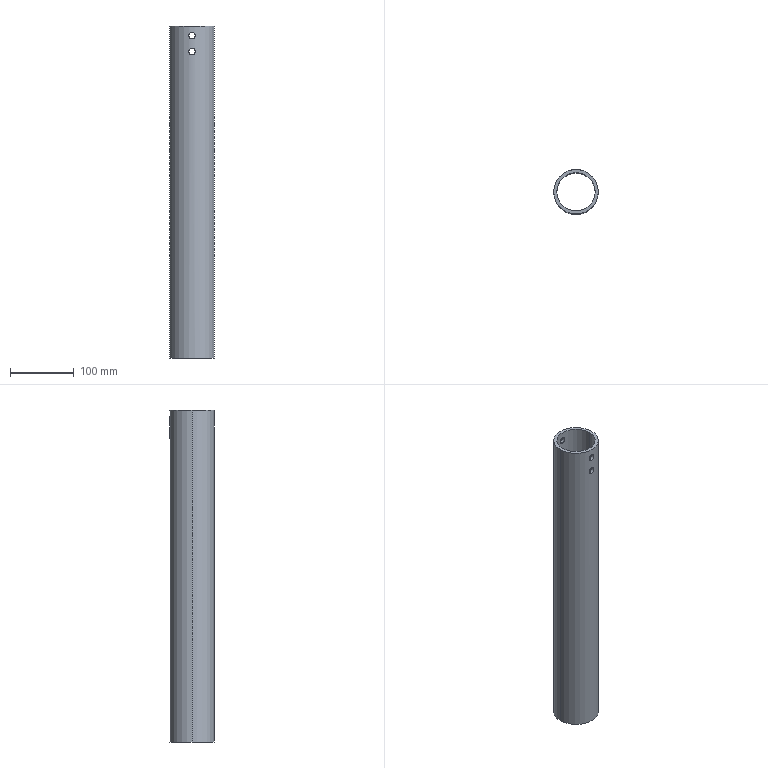Part | SolidWorks | features ICE 4, Cut 1, Extrusion 1 | 1 solid | 14 faces | box 70 x 70 x 520 mm | volume 529289 mm3 | cylinder 12 | plane 2 | commonest cylinder face diameters 10.2 x8 60 x2 70 x2
STEP:
#1=CARTESIAN_POINT('',(0.,-35.,499.9));
#2=VERTEX_POINT('',#1);
#3=CARTESIAN_POINT('',(0.,-35.,510.1));
#4=VERTEX_POINT('',#3);
#5=CARTESIAN_POINT('',(0.,-35.,499.9));
#6=CARTESIAN_POINT('',(-0.333,-35.,499.9));
#7=CARTESIAN_POINT('',(-0.6643,-34.995,499.932));
#8=CARTESIAN_POINT('',(-1.323,-34.977,500.063));
#9=CARTESIAN_POINT('',(-1.645,-34.963,500.161));
#10=CARTESIAN_POINT('',(-2.259,-34.928,500.415));
#11=CARTESIAN_POINT('',(-2.556,-34.908,500.574));
#12=CARTESIAN_POINT('',(-3.112,-34.862,500.946));
#13=CARTESIAN_POINT('',(-3.369,-34.838,501.157));
#14=CARTESIAN_POINT('',(-3.839,-34.79,501.626));
#15=CARTESIAN_POINT('',(-4.054,-34.765,501.888));
#16=CARTESIAN_POINT('',(-4.424,-34.72,502.441));
#17=CARTESIAN_POINT('',(-4.581,-34.699,502.734));
#18=CARTESIAN_POINT('',(-4.774,-34.673,503.197));
#19=CARTESIAN_POINT('',(-4.831,-34.665,503.356));
#20=CARTESIAN_POINT('',(-4.928,-34.651,503.677));
#21=CARTESIAN_POINT('',(-4.969,-34.646,503.838));
#22=CARTESIAN_POINT('',(-5.066,-34.631,504.327));
#23=CARTESIAN_POINT('',(-5.1,-34.626,504.66));
#24=CARTESIAN_POINT('',(-5.1,-34.626,505.334));
#25=CARTESIAN_POINT('',(-5.067,-34.631,505.665));
#26=CARTESIAN_POINT('',(-4.938,-34.65,506.318));
#27=CARTESIAN_POINT('',(-4.84,-34.664,506.642));
#28=CARTESIAN_POINT('',(-4.584,-34.699,507.259));
#29=CARTESIAN_POINT('',(-4.428,-34.719,507.552));
#30=CARTESIAN_POINT('',(-4.058,-34.764,508.107));
#31=CARTESIAN_POINT('',(-3.843,-34.789,508.369));
#32=CARTESIAN_POINT('',(-3.374,-34.838,508.839));
#33=CARTESIAN_POINT('',(-3.118,-34.862,509.05));
#34=CARTESIAN_POINT('',(-2.56,-34.907,509.424));
#35=CARTESIAN_POINT('',(-2.265,-34.928,509.582));
#36=CARTESIAN_POINT('',(-1.652,-34.962,509.837));
#37=CARTESIAN_POINT('',(-1.33,-34.976,509.935));
#38=CARTESIAN_POINT('',(-0.6708,-34.995,510.067));
#39=CARTESIAN_POINT('',(-0.3374,-35.,510.1));
#40=CARTESIAN_POINT('',(0.,-35.,510.1));
#41=B_SPLINE_CURVE_WITH_KNOTS('',3,(#5,#6,#7,#8,#9,#10,#11,#12,#13,#14,#15,#16,#17,#18,#19,#20,#21,#22,#23,#24,#25,#26,#27,#28,#29,#30,#31,#32,#33,#34,#35,#36,#37,#38,#39,#40),.UNSPECIFIED.,.F.,.F.,(4,2,2,2,2,2,2,2,2,2,2,2,2,2,2,2,2,4),(0.01597,0.01696,0.01796,0.01896,0.01996,0.02095,0.02195,0.02245,0.02295,0.02395,0.02494,0.02594,0.02694,0.02794,0.02894,0.02993,0.03093,0.03193),.UNSPECIFIED.);
#42=EDGE_CURVE('',#2,#4,#41,.T.);
#43=ORIENTED_EDGE('',*,*,#42,.F.);
#44=CARTESIAN_POINT('',(0.,-30.,499.9));
#45=VERTEX_POINT('',#44);
#46=CARTESIAN_POINT('',(0.,-91.,499.9));
#47=DIRECTION('',(0.,1.,0.));
#48=VECTOR('',#47,1000.);
#49=LINE('',#46,#48);
#50=EDGE_CURVE('',#2,#45,#49,.T.);
#51=ORIENTED_EDGE('',*,*,#50,.T.);
#52=CARTESIAN_POINT('',(0.,-30.,510.1));
#53=VERTEX_POINT('',#52);
#54=CARTESIAN_POINT('',(0.,-30.,499.9));
#55=CARTESIAN_POINT('',(-0.3331,-30.,499.9));
#56=CARTESIAN_POINT('',(-0.6646,-29.994,499.932));
#57=CARTESIAN_POINT('',(-1.324,-29.973,500.063));
#58=CARTESIAN_POINT('',(-1.645,-29.956,500.161));
#59=CARTESIAN_POINT('',(-2.106,-29.926,500.352));
#60=CARTESIAN_POINT('',(-2.256,-29.915,500.423));
#61=CARTESIAN_POINT('',(-2.551,-29.892,500.58));
#62=CARTESIAN_POINT('',(-2.696,-29.879,500.667));
#63=CARTESIAN_POINT('',(-3.112,-29.839,500.946));
#64=CARTESIAN_POINT('',(-3.369,-29.811,501.157));
#65=CARTESIAN_POINT('',(-3.839,-29.754,501.626));
#66=CARTESIAN_POINT('',(-4.054,-29.725,501.888));
#67=CARTESIAN_POINT('',(-4.424,-29.673,502.441));
#68=CARTESIAN_POINT('',(-4.581,-29.648,502.733));
#69=CARTESIAN_POINT('',(-4.774,-29.618,503.197));
#70=CARTESIAN_POINT('',(-4.831,-29.609,503.356));
#71=CARTESIAN_POINT('',(-4.928,-29.593,503.676));
#72=CARTESIAN_POINT('',(-4.969,-29.586,503.838));
#73=CARTESIAN_POINT('',(-5.066,-29.569,504.327));
#74=CARTESIAN_POINT('',(-5.1,-29.563,504.66));
#75=CARTESIAN_POINT('',(-5.1,-29.563,505.334));
#76=CARTESIAN_POINT('',(-5.067,-29.569,505.665));
#77=CARTESIAN_POINT('',(-4.938,-29.591,506.318));
#78=CARTESIAN_POINT('',(-4.84,-29.607,506.643));
#79=CARTESIAN_POINT('',(-4.584,-29.648,507.26));
#80=CARTESIAN_POINT('',(-4.428,-29.672,507.553));
#81=CARTESIAN_POINT('',(-4.058,-29.725,508.108));
#82=CARTESIAN_POINT('',(-3.843,-29.754,508.369));
#83=CARTESIAN_POINT('',(-3.374,-29.811,508.839));
#84=CARTESIAN_POINT('',(-3.118,-29.839,509.05));
#85=CARTESIAN_POINT('',(-2.56,-29.892,509.424));
#86=CARTESIAN_POINT('',(-2.265,-29.916,509.581));
#87=CARTESIAN_POINT('',(-1.652,-29.956,509.836));
#88=CARTESIAN_POINT('',(-1.33,-29.972,509.935));
#89=CARTESIAN_POINT('',(-0.6709,-29.994,510.067));
#90=CARTESIAN_POINT('',(-0.3375,-30.,510.1));
#91=CARTESIAN_POINT('',(0.,-30.,510.1));
#92=B_SPLINE_CURVE_WITH_KNOTS('',3,(#54,#55,#56,#57,#58,#59,#60,#61,#62,#63,#64,#65,#66,#67,#68,#69,#70,#71,#72,#73,#74,#75,#76,#77,#78,#79,#80,#81,#82,#83,#84,#85,#86,#87,#88,#89,#90,#91),.UNSPECIFIED.,.F.,.F.,(4,2,2,2,2,2,2,2,2,2,2,2,2,2,2,2,2,2,4),(0.01597,0.01697,0.01797,0.01847,0.01897,0.01997,0.02096,0.02196,0.02246,0.02296,0.02396,0.02496,0.02596,0.02695,0.02795,0.02895,0.02995,0.03095,0.03194),.UNSPECIFIED.);
#93=EDGE_CURVE('',#45,#53,#92,.T.);
#94=ORIENTED_EDGE('',*,*,#93,.T.);
#95=CARTESIAN_POINT('',(0.,-91.,510.1));
#96=DIRECTION('',(0.,1.,0.));
#97=VECTOR('',#96,1000.);
#98=LINE('',#95,#97);
#99=EDGE_CURVE('',#4,#53,#98,.T.);
#100=ORIENTED_EDGE('',*,*,#99,.F.);
#101=EDGE_LOOP('',(#43,#51,#94,#100));
#102=FACE_OUTER_BOUND('',#101,.T.);
#103=CARTESIAN_POINT('',(0.,-91.,505.));
#104=DIRECTION('',(0.,1.,0.));
#105=DIRECTION('',(0.,0.,1.));
#106=AXIS2_PLACEMENT_3D('',#103,#104,#105);
#107=CYLINDRICAL_SURFACE('',#106,5.1);
#108=ADVANCED_FACE('',(#102),#107,.F.);
#109=CARTESIAN_POINT('',(0.,30.,510.1));
#110=VERTEX_POINT('',#109);
#111=CARTESIAN_POINT('',(0.,30.,499.9));
#112=VERTEX_POINT('',#111);
#113=CARTESIAN_POINT('',(0.,30.,510.1));
#114=CARTESIAN_POINT('',(-0.3376,30.,510.1));
#115=CARTESIAN_POINT('',(-0.6695,29.994,510.067));
#116=CARTESIAN_POINT('',(-1.159,29.978,509.969));
#117=CARTESIAN_POINT('',(-1.321,29.971,509.929));
#118=CARTESIAN_POINT('',(-1.642,29.955,509.831));
#119=CARTESIAN_POINT('',(-1.801,29.946,509.774));
#120=CARTESIAN_POINT('',(-2.264,29.916,509.582));
#121=CARTESIAN_POINT('',(-2.557,29.892,509.425));
#122=CARTESIAN_POINT('',(-3.111,29.84,509.055));
#123=CARTESIAN_POINT('',(-3.372,29.811,508.84));
#124=CARTESIAN_POINT('',(-3.842,29.754,508.371));
#125=CARTESIAN_POINT('',(-4.053,29.726,508.114));
#126=CARTESIAN_POINT('',(-4.426,29.672,507.557));
#127=CARTESIAN_POINT('',(-4.584,29.648,507.261));
#128=CARTESIAN_POINT('',(-4.838,29.608,506.647));
#129=CARTESIAN_POINT('',(-4.936,29.591,506.325));
#130=CARTESIAN_POINT('',(-5.067,29.569,505.667));
#131=CARTESIAN_POINT('',(-5.1,29.563,505.335));
#132=CARTESIAN_POINT('',(-5.1,29.563,504.669));
#133=CARTESIAN_POINT('',(-5.067,29.569,504.33));
#134=CARTESIAN_POINT('',(-4.936,29.591,503.675));
#135=CARTESIAN_POINT('',(-4.84,29.607,503.357));
#136=CARTESIAN_POINT('',(-4.648,29.638,502.893));
#137=CARTESIAN_POINT('',(-4.575,29.649,502.741));
#138=CARTESIAN_POINT('',(-4.418,29.673,502.446));
#139=CARTESIAN_POINT('',(-4.332,29.686,502.303));
#140=CARTESIAN_POINT('',(-4.055,29.725,501.889));
#141=CARTESIAN_POINT('',(-3.844,29.754,501.631));
#142=CARTESIAN_POINT('',(-3.369,29.811,501.156));
#143=CARTESIAN_POINT('',(-3.112,29.839,500.946));
#144=CARTESIAN_POINT('',(-2.56,29.892,500.577));
#145=CARTESIAN_POINT('',(-2.261,29.916,500.417));
#146=CARTESIAN_POINT('',(-1.645,29.956,500.161));
#147=CARTESIAN_POINT('',(-1.327,29.972,500.064));
#148=CARTESIAN_POINT('',(-0.6716,29.994,499.933));
#149=CARTESIAN_POINT('',(-0.3332,30.,499.9));
#150=CARTESIAN_POINT('',(0.,30.,499.9));
#151=B_SPLINE_CURVE_WITH_KNOTS('',3,(#113,#114,#115,#116,#117,#118,#119,#120,#121,#122,#123,#124,#125,#126,#127,#128,#129,#130,#131,#132,#133,#134,#135,#136,#137,#138,#139,#140,#141,#142,#143,#144,#145,#146,#147,#148,#149,#150),.UNSPECIFIED.,.F.,.F.,(4,2,2,2,2,2,2,2,2,2,2,2,2,2,2,2,2,2,4),(0.,0.0009984,0.001498,0.001997,0.002995,0.003993,0.004992,0.00599,0.006989,0.007987,0.008985,0.009984,0.01048,0.01098,0.01198,0.01298,0.01398,0.01498,0.01597),.UNSPECIFIED.);
#152=EDGE_CURVE('',#110,#112,#151,.T.);
#153=ORIENTED_EDGE('',*,*,#152,.T.);
#154=CARTESIAN_POINT('',(0.,35.,499.9));
#155=VERTEX_POINT('',#154);
#156=CARTESIAN_POINT('',(0.,-91.,499.9));
#157=DIRECTION('',(0.,1.,0.));
#158=VECTOR('',#157,1000.);
#159=LINE('',#156,#158);
#160=EDGE_CURVE('',#112,#155,#159,.T.);
#161=ORIENTED_EDGE('',*,*,#160,.T.);
#162=CARTESIAN_POINT('',(0.,35.,510.1));
#163=VERTEX_POINT('',#162);
#164=CARTESIAN_POINT('',(0.,35.,510.1));
#165=CARTESIAN_POINT('',(-0.3375,35.,510.1));
#166=CARTESIAN_POINT('',(-0.6692,34.995,510.067));
#167=CARTESIAN_POINT('',(-1.159,34.981,509.969));
#168=CARTESIAN_POINT('',(-1.32,34.975,509.929));
#169=CARTESIAN_POINT('',(-1.641,34.962,509.832));
#170=CARTESIAN_POINT('',(-1.8,34.954,509.775));
#171=CARTESIAN_POINT('',(-2.263,34.928,509.582));
#172=CARTESIAN_POINT('',(-2.556,34.908,509.426));
#173=CARTESIAN_POINT('',(-3.11,34.863,509.056));
#174=CARTESIAN_POINT('',(-3.372,34.838,508.84));
#175=CARTESIAN_POINT('',(-3.842,34.789,508.371));
#176=CARTESIAN_POINT('',(-4.053,34.765,508.114));
#177=CARTESIAN_POINT('',(-4.426,34.72,507.557));
#178=CARTESIAN_POINT('',(-4.584,34.699,507.26));
#179=CARTESIAN_POINT('',(-4.838,34.664,506.647));
#180=CARTESIAN_POINT('',(-4.936,34.65,506.325));
#181=CARTESIAN_POINT('',(-5.067,34.631,505.666));
#182=CARTESIAN_POINT('',(-5.1,34.626,505.335));
#183=CARTESIAN_POINT('',(-5.1,34.626,504.669));
#184=CARTESIAN_POINT('',(-5.067,34.631,504.33));
#185=CARTESIAN_POINT('',(-4.936,34.65,503.676));
#186=CARTESIAN_POINT('',(-4.84,34.664,503.358));
#187=CARTESIAN_POINT('',(-4.648,34.69,502.894));
#188=CARTESIAN_POINT('',(-4.576,34.7,502.741));
#189=CARTESIAN_POINT('',(-4.418,34.72,502.446));
#190=CARTESIAN_POINT('',(-4.332,34.731,502.304));
#191=CARTESIAN_POINT('',(-4.055,34.765,501.89));
#192=CARTESIAN_POINT('',(-3.844,34.789,501.632));
#193=CARTESIAN_POINT('',(-3.369,34.838,501.156));
#194=CARTESIAN_POINT('',(-3.112,34.863,500.946));
#195=CARTESIAN_POINT('',(-2.698,34.896,500.669));
#196=CARTESIAN_POINT('',(-2.555,34.907,500.583));
#197=CARTESIAN_POINT('',(-2.26,34.927,500.425));
#198=CARTESIAN_POINT('',(-2.107,34.937,500.353));
#199=CARTESIAN_POINT('',(-1.644,34.963,500.161));
#200=CARTESIAN_POINT('',(-1.326,34.976,500.064));
#201=CARTESIAN_POINT('',(-0.6714,34.995,499.933));
#202=CARTESIAN_POINT('',(-0.3331,35.,499.9));
#203=CARTESIAN_POINT('',(0.,35.,499.9));
#204=B_SPLINE_CURVE_WITH_KNOTS('',3,(#164,#165,#166,#167,#168,#169,#170,#171,#172,#173,#174,#175,#176,#177,#178,#179,#180,#181,#182,#183,#184,#185,#186,#187,#188,#189,#190,#191,#192,#193,#194,#195,#196,#197,#198,#199,#200,#201,#202,#203),.UNSPECIFIED.,.F.,.F.,(4,2,2,2,2,2,2,2,2,2,2,2,2,2,2,2,2,2,2,4),(0.,0.0009979,0.001497,0.001996,0.002994,0.003992,0.004989,0.005987,0.006985,0.007983,0.008981,0.009979,0.01048,0.01098,0.01197,0.01297,0.01347,0.01397,0.01497,0.01597),.UNSPECIFIED.);
#205=EDGE_CURVE('',#163,#155,#204,.T.);
#206=ORIENTED_EDGE('',*,*,#205,.F.);
#207=CARTESIAN_POINT('',(0.,-91.,510.1));
#208=DIRECTION('',(0.,1.,0.));
#209=VECTOR('',#208,1000.);
#210=LINE('',#207,#209);
#211=EDGE_CURVE('',#110,#163,#210,.T.);
#212=ORIENTED_EDGE('',*,*,#211,.F.);
#213=EDGE_LOOP('',(#153,#161,#206,#212));
#214=FACE_OUTER_BOUND('',#213,.T.);
#215=CARTESIAN_POINT('',(0.,-91.,505.));
#216=DIRECTION('',(0.,1.,0.));
#217=DIRECTION('',(0.,0.,1.));
#218=AXIS2_PLACEMENT_3D('',#215,#216,#217);
#219=CYLINDRICAL_SURFACE('',#218,5.1);
#220=ADVANCED_FACE('',(#214),#219,.F.);
#221=CARTESIAN_POINT('',(0.,-35.,474.9));
#222=VERTEX_POINT('',#221);
#223=CARTESIAN_POINT('',(0.,-35.,485.1));
#224=VERTEX_POINT('',#223);
#225=CARTESIAN_POINT('',(0.,-35.,474.9));
#226=CARTESIAN_POINT('',(-0.333,-35.,474.9));
#227=CARTESIAN_POINT('',(-0.6643,-34.995,474.932));
#228=CARTESIAN_POINT('',(-1.323,-34.977,475.063));
#229=CARTESIAN_POINT('',(-1.645,-34.963,475.161));
#230=CARTESIAN_POINT('',(-2.259,-34.928,475.415));
#231=CARTESIAN_POINT('',(-2.556,-34.908,475.574));
#232=CARTESIAN_POINT('',(-3.112,-34.862,475.946));
#233=CARTESIAN_POINT('',(-3.369,-34.838,476.157));
#234=CARTESIAN_POINT('',(-3.839,-34.79,476.626));
#235=CARTESIAN_POINT('',(-4.054,-34.765,476.888));
#236=CARTESIAN_POINT('',(-4.424,-34.72,477.441));
#237=CARTESIAN_POINT('',(-4.581,-34.699,477.734));
#238=CARTESIAN_POINT('',(-4.774,-34.673,478.197));
#239=CARTESIAN_POINT('',(-4.831,-34.665,478.356));
#240=CARTESIAN_POINT('',(-4.928,-34.651,478.677));
#241=CARTESIAN_POINT('',(-4.969,-34.646,478.838));
#242=CARTESIAN_POINT('',(-5.066,-34.631,479.327));
#243=CARTESIAN_POINT('',(-5.1,-34.626,479.66));
#244=CARTESIAN_POINT('',(-5.1,-34.626,480.334));
#245=CARTESIAN_POINT('',(-5.067,-34.631,480.665));
#246=CARTESIAN_POINT('',(-4.938,-34.65,481.318));
#247=CARTESIAN_POINT('',(-4.84,-34.664,481.642));
#248=CARTESIAN_POINT('',(-4.584,-34.699,482.259));
#249=CARTESIAN_POINT('',(-4.428,-34.719,482.552));
#250=CARTESIAN_POINT('',(-4.058,-34.764,483.107));
#251=CARTESIAN_POINT('',(-3.843,-34.789,483.369));
#252=CARTESIAN_POINT('',(-3.374,-34.838,483.839));
#253=CARTESIAN_POINT('',(-3.118,-34.862,484.05));
#254=CARTESIAN_POINT('',(-2.56,-34.907,484.424));
#255=CARTESIAN_POINT('',(-2.265,-34.928,484.582));
#256=CARTESIAN_POINT('',(-1.652,-34.962,484.837));
#257=CARTESIAN_POINT('',(-1.33,-34.976,484.935));
#258=CARTESIAN_POINT('',(-0.6708,-34.995,485.067));
#259=CARTESIAN_POINT('',(-0.3374,-35.,485.1));
#260=CARTESIAN_POINT('',(0.,-35.,485.1));
#261=B_SPLINE_CURVE_WITH_KNOTS('',3,(#225,#226,#227,#228,#229,#230,#231,#232,#233,#234,#235,#236,#237,#238,#239,#240,#241,#242,#243,#244,#245,#246,#247,#248,#249,#250,#251,#252,#253,#254,#255,#256,#257,#258,#259,#260),.UNSPECIFIED.,.F.,.F.,(4,2,2,2,2,2,2,2,2,2,2,2,2,2,2,2,2,4),(0.01597,0.01696,0.01796,0.01896,0.01996,0.02095,0.02195,0.02245,0.02295,0.02395,0.02494,0.02594,0.02694,0.02794,0.02894,0.02993,0.03093,0.03193),.UNSPECIFIED.);
#262=EDGE_CURVE('',#222,#224,#261,.T.);
#263=ORIENTED_EDGE('',*,*,#262,.F.);
#264=CARTESIAN_POINT('',(0.,-30.,474.9));
#265=VERTEX_POINT('',#264);
#266=CARTESIAN_POINT('',(0.,-91.,474.9));
#267=DIRECTION('',(0.,1.,0.));
#268=VECTOR('',#267,1000.);
#269=LINE('',#266,#268);
#270=EDGE_CURVE('',#222,#265,#269,.T.);
#271=ORIENTED_EDGE('',*,*,#270,.T.);
#272=CARTESIAN_POINT('',(0.,-30.,485.1));
#273=VERTEX_POINT('',#272);
#274=CARTESIAN_POINT('',(0.,-30.,474.9));
#275=CARTESIAN_POINT('',(-0.3331,-30.,474.9));
#276=CARTESIAN_POINT('',(-0.6646,-29.994,474.932));
#277=CARTESIAN_POINT('',(-1.324,-29.973,475.063));
#278=CARTESIAN_POINT('',(-1.645,-29.956,475.161));
#279=CARTESIAN_POINT('',(-2.106,-29.926,475.352));
#280=CARTESIAN_POINT('',(-2.256,-29.915,475.423));
#281=CARTESIAN_POINT('',(-2.551,-29.892,475.58));
#282=CARTESIAN_POINT('',(-2.696,-29.879,475.667));
#283=CARTESIAN_POINT('',(-3.112,-29.839,475.946));
#284=CARTESIAN_POINT('',(-3.369,-29.811,476.157));
#285=CARTESIAN_POINT('',(-3.839,-29.754,476.626));
#286=CARTESIAN_POINT('',(-4.054,-29.725,476.888));
#287=CARTESIAN_POINT('',(-4.424,-29.673,477.441));
#288=CARTESIAN_POINT('',(-4.581,-29.648,477.733));
#289=CARTESIAN_POINT('',(-4.774,-29.618,478.197));
#290=CARTESIAN_POINT('',(-4.831,-29.609,478.356));
#291=CARTESIAN_POINT('',(-4.928,-29.593,478.676));
#292=CARTESIAN_POINT('',(-4.969,-29.586,478.838));
#293=CARTESIAN_POINT('',(-5.066,-29.569,479.327));
#294=CARTESIAN_POINT('',(-5.1,-29.563,479.66));
#295=CARTESIAN_POINT('',(-5.1,-29.563,480.334));
#296=CARTESIAN_POINT('',(-5.067,-29.569,480.665));
#297=CARTESIAN_POINT('',(-4.938,-29.591,481.318));
#298=CARTESIAN_POINT('',(-4.84,-29.607,481.643));
#299=CARTESIAN_POINT('',(-4.584,-29.648,482.26));
#300=CARTESIAN_POINT('',(-4.428,-29.672,482.553));
#301=CARTESIAN_POINT('',(-4.058,-29.725,483.108));
#302=CARTESIAN_POINT('',(-3.843,-29.754,483.369));
#303=CARTESIAN_POINT('',(-3.374,-29.811,483.839));
#304=CARTESIAN_POINT('',(-3.118,-29.839,484.05));
#305=CARTESIAN_POINT('',(-2.56,-29.892,484.424));
#306=CARTESIAN_POINT('',(-2.265,-29.916,484.581));
#307=CARTESIAN_POINT('',(-1.652,-29.956,484.836));
#308=CARTESIAN_POINT('',(-1.33,-29.972,484.935));
#309=CARTESIAN_POINT('',(-0.6709,-29.994,485.067));
#310=CARTESIAN_POINT('',(-0.3375,-30.,485.1));
#311=CARTESIAN_POINT('',(0.,-30.,485.1));
#312=B_SPLINE_CURVE_WITH_KNOTS('',3,(#274,#275,#276,#277,#278,#279,#280,#281,#282,#283,#284,#285,#286,#287,#288,#289,#290,#291,#292,#293,#294,#295,#296,#297,#298,#299,#300,#301,#302,#303,#304,#305,#306,#307,#308,#309,#310,#311),.UNSPECIFIED.,.F.,.F.,(4,2,2,2,2,2,2,2,2,2,2,2,2,2,2,2,2,2,4),(0.01597,0.01697,0.01797,0.01847,0.01897,0.01997,0.02096,0.02196,0.02246,0.02296,0.02396,0.02496,0.02596,0.02695,0.02795,0.02895,0.02995,0.03095,0.03194),.UNSPECIFIED.);
#313=EDGE_CURVE('',#265,#273,#312,.T.);
#314=ORIENTED_EDGE('',*,*,#313,.T.);
#315=CARTESIAN_POINT('',(0.,-91.,485.1));
#316=DIRECTION('',(0.,1.,0.));
#317=VECTOR('',#316,1000.);
#318=LINE('',#315,#317);
#319=EDGE_CURVE('',#224,#273,#318,.T.);
#320=ORIENTED_EDGE('',*,*,#319,.F.);
#321=EDGE_LOOP('',(#263,#271,#314,#320));
#322=FACE_OUTER_BOUND('',#321,.T.);
#323=CARTESIAN_POINT('',(0.,-91.,480.));
#324=DIRECTION('',(0.,1.,0.));
#325=DIRECTION('',(0.,0.,1.));
#326=AXIS2_PLACEMENT_3D('',#323,#324,#325);
#327=CYLINDRICAL_SURFACE('',#326,5.1);
#328=ADVANCED_FACE('',(#322),#327,.F.);
#329=CARTESIAN_POINT('',(0.,30.,485.1));
#330=VERTEX_POINT('',#329);
#331=CARTESIAN_POINT('',(0.,30.,474.9));
#332=VERTEX_POINT('',#331);
#333=CARTESIAN_POINT('',(0.,30.,485.1));
#334=CARTESIAN_POINT('',(-0.3376,30.,485.1));
#335=CARTESIAN_POINT('',(-0.6695,29.994,485.067));
#336=CARTESIAN_POINT('',(-1.159,29.978,484.969));
#337=CARTESIAN_POINT('',(-1.321,29.971,484.929));
#338=CARTESIAN_POINT('',(-1.642,29.955,484.831));
#339=CARTESIAN_POINT('',(-1.801,29.946,484.774));
#340=CARTESIAN_POINT('',(-2.264,29.916,484.582));
#341=CARTESIAN_POINT('',(-2.557,29.892,484.425));
#342=CARTESIAN_POINT('',(-3.111,29.84,484.055));
#343=CARTESIAN_POINT('',(-3.372,29.811,483.84));
#344=CARTESIAN_POINT('',(-3.842,29.754,483.371));
#345=CARTESIAN_POINT('',(-4.053,29.726,483.114));
#346=CARTESIAN_POINT('',(-4.426,29.672,482.557));
#347=CARTESIAN_POINT('',(-4.584,29.648,482.261));
#348=CARTESIAN_POINT('',(-4.838,29.608,481.647));
#349=CARTESIAN_POINT('',(-4.936,29.591,481.325));
#350=CARTESIAN_POINT('',(-5.067,29.569,480.667));
#351=CARTESIAN_POINT('',(-5.1,29.563,480.335));
#352=CARTESIAN_POINT('',(-5.1,29.563,479.669));
#353=CARTESIAN_POINT('',(-5.067,29.569,479.33));
#354=CARTESIAN_POINT('',(-4.936,29.591,478.675));
#355=CARTESIAN_POINT('',(-4.84,29.607,478.357));
#356=CARTESIAN_POINT('',(-4.648,29.638,477.893));
#357=CARTESIAN_POINT('',(-4.575,29.649,477.741));
#358=CARTESIAN_POINT('',(-4.418,29.673,477.446));
#359=CARTESIAN_POINT('',(-4.332,29.686,477.303));
#360=CARTESIAN_POINT('',(-4.055,29.725,476.889));
#361=CARTESIAN_POINT('',(-3.844,29.754,476.631));
#362=CARTESIAN_POINT('',(-3.369,29.811,476.156));
#363=CARTESIAN_POINT('',(-3.112,29.839,475.946));
#364=CARTESIAN_POINT('',(-2.56,29.892,475.577));
#365=CARTESIAN_POINT('',(-2.261,29.916,475.417));
#366=CARTESIAN_POINT('',(-1.645,29.956,475.161));
#367=CARTESIAN_POINT('',(-1.327,29.972,475.064));
#368=CARTESIAN_POINT('',(-0.6716,29.994,474.933));
#369=CARTESIAN_POINT('',(-0.3332,30.,474.9));
#370=CARTESIAN_POINT('',(0.,30.,474.9));
#371=B_SPLINE_CURVE_WITH_KNOTS('',3,(#333,#334,#335,#336,#337,#338,#339,#340,#341,#342,#343,#344,#345,#346,#347,#348,#349,#350,#351,#352,#353,#354,#355,#356,#357,#358,#359,#360,#361,#362,#363,#364,#365,#366,#367,#368,#369,#370),.UNSPECIFIED.,.F.,.F.,(4,2,2,2,2,2,2,2,2,2,2,2,2,2,2,2,2,2,4),(0.,0.0009984,0.001498,0.001997,0.002995,0.003993,0.004992,0.00599,0.006989,0.007987,0.008985,0.009984,0.01048,0.01098,0.01198,0.01298,0.01398,0.01498,0.01597),.UNSPECIFIED.);
#372=EDGE_CURVE('',#330,#332,#371,.T.);
#373=ORIENTED_EDGE('',*,*,#372,.T.);
#374=CARTESIAN_POINT('',(0.,35.,474.9));
#375=VERTEX_POINT('',#374);
#376=CARTESIAN_POINT('',(0.,-91.,474.9));
#377=DIRECTION('',(0.,1.,0.));
#378=VECTOR('',#377,1000.);
#379=LINE('',#376,#378);
#380=EDGE_CURVE('',#332,#375,#379,.T.);
#381=ORIENTED_EDGE('',*,*,#380,.T.);
#382=CARTESIAN_POINT('',(0.,35.,485.1));
#383=VERTEX_POINT('',#382);
#384=CARTESIAN_POINT('',(0.,35.,485.1));
#385=CARTESIAN_POINT('',(-0.3375,35.,485.1));
#386=CARTESIAN_POINT('',(-0.6692,34.995,485.067));
#387=CARTESIAN_POINT('',(-1.159,34.981,484.969));
#388=CARTESIAN_POINT('',(-1.32,34.975,484.929));
#389=CARTESIAN_POINT('',(-1.641,34.962,484.832));
#390=CARTESIAN_POINT('',(-1.8,34.954,484.775));
#391=CARTESIAN_POINT('',(-2.263,34.928,484.582));
#392=CARTESIAN_POINT('',(-2.556,34.908,484.426));
#393=CARTESIAN_POINT('',(-3.11,34.863,484.056));
#394=CARTESIAN_POINT('',(-3.372,34.838,483.84));
#395=CARTESIAN_POINT('',(-3.842,34.789,483.371));
#396=CARTESIAN_POINT('',(-4.053,34.765,483.114));
#397=CARTESIAN_POINT('',(-4.426,34.72,482.557));
#398=CARTESIAN_POINT('',(-4.584,34.699,482.26));
#399=CARTESIAN_POINT('',(-4.838,34.664,481.647));
#400=CARTESIAN_POINT('',(-4.936,34.65,481.325));
#401=CARTESIAN_POINT('',(-5.067,34.631,480.666));
#402=CARTESIAN_POINT('',(-5.1,34.626,480.335));
#403=CARTESIAN_POINT('',(-5.1,34.626,479.669));
#404=CARTESIAN_POINT('',(-5.067,34.631,479.33));
#405=CARTESIAN_POINT('',(-4.936,34.65,478.676));
#406=CARTESIAN_POINT('',(-4.84,34.664,478.358));
#407=CARTESIAN_POINT('',(-4.648,34.69,477.894));
#408=CARTESIAN_POINT('',(-4.576,34.7,477.741));
#409=CARTESIAN_POINT('',(-4.418,34.72,477.446));
#410=CARTESIAN_POINT('',(-4.332,34.731,477.304));
#411=CARTESIAN_POINT('',(-4.055,34.765,476.89));
#412=CARTESIAN_POINT('',(-3.844,34.789,476.632));
#413=CARTESIAN_POINT('',(-3.369,34.838,476.156));
#414=CARTESIAN_POINT('',(-3.112,34.863,475.946));
#415=CARTESIAN_POINT('',(-2.698,34.896,475.669));
#416=CARTESIAN_POINT('',(-2.555,34.907,475.583));
#417=CARTESIAN_POINT('',(-2.26,34.927,475.425));
#418=CARTESIAN_POINT('',(-2.107,34.937,475.353));
#419=CARTESIAN_POINT('',(-1.644,34.963,475.161));
#420=CARTESIAN_POINT('',(-1.326,34.976,475.064));
#421=CARTESIAN_POINT('',(-0.6714,34.995,474.933));
#422=CARTESIAN_POINT('',(-0.3331,35.,474.9));
#423=CARTESIAN_POINT('',(0.,35.,474.9));
#424=B_SPLINE_CURVE_WITH_KNOTS('',3,(#384,#385,#386,#387,#388,#389,#390,#391,#392,#393,#394,#395,#396,#397,#398,#399,#400,#401,#402,#403,#404,#405,#406,#407,#408,#409,#410,#411,#412,#413,#414,#415,#416,#417,#418,#419,#420,#421,#422,#423),.UNSPECIFIED.,.F.,.F.,(4,2,2,2,2,2,2,2,2,2,2,2,2,2,2,2,2,2,2,4),(0.,0.0009979,0.001497,0.001996,0.002994,0.003992,0.004989,0.005987,0.006985,0.007983,0.008981,0.009979,0.01048,0.01098,0.01197,0.01297,0.01347,0.01397,0.01497,0.01597),.UNSPECIFIED.);
#425=EDGE_CURVE('',#383,#375,#424,.T.);
#426=ORIENTED_EDGE('',*,*,#425,.F.);
#427=CARTESIAN_POINT('',(0.,-91.,485.1));
#428=DIRECTION('',(0.,1.,0.));
#429=VECTOR('',#428,1000.);
#430=LINE('',#427,#429);
#431=EDGE_CURVE('',#330,#383,#430,.T.);
#432=ORIENTED_EDGE('',*,*,#431,.F.);
#433=EDGE_LOOP('',(#373,#381,#426,#432));
#434=FACE_OUTER_BOUND('',#433,.T.);
#435=CARTESIAN_POINT('',(0.,-91.,480.));
#436=DIRECTION('',(0.,1.,0.));
#437=DIRECTION('',(0.,0.,1.));
#438=AXIS2_PLACEMENT_3D('',#435,#436,#437);
#439=CYLINDRICAL_SURFACE('',#438,5.1);
#440=ADVANCED_FACE('',(#434),#439,.F.);
#441=CARTESIAN_POINT('',(0.,-30.,485.1));
#442=CARTESIAN_POINT('',(0.3376,-30.,485.1));
#443=CARTESIAN_POINT('',(0.6695,-29.994,485.067));
#444=CARTESIAN_POINT('',(1.159,-29.978,484.969));
#445=CARTESIAN_POINT('',(1.321,-29.971,484.929));
#446=CARTESIAN_POINT('',(1.642,-29.955,484.831));
#447=CARTESIAN_POINT('',(1.801,-29.946,484.774));
#448=CARTESIAN_POINT('',(2.264,-29.916,484.582));
#449=CARTESIAN_POINT('',(2.557,-29.892,484.425));
#450=CARTESIAN_POINT('',(3.111,-29.84,484.055));
#451=CARTESIAN_POINT('',(3.372,-29.811,483.84));
#452=CARTESIAN_POINT('',(3.842,-29.754,483.371));
#453=CARTESIAN_POINT('',(4.053,-29.726,483.114));
#454=CARTESIAN_POINT('',(4.426,-29.672,482.557));
#455=CARTESIAN_POINT('',(4.584,-29.648,482.261));
#456=CARTESIAN_POINT('',(4.838,-29.608,481.647));
#457=CARTESIAN_POINT('',(4.936,-29.591,481.325));
#458=CARTESIAN_POINT('',(5.067,-29.569,480.667));
#459=CARTESIAN_POINT('',(5.1,-29.563,480.335));
#460=CARTESIAN_POINT('',(5.1,-29.563,479.669));
#461=CARTESIAN_POINT('',(5.067,-29.569,479.33));
#462=CARTESIAN_POINT('',(4.936,-29.591,478.675));
#463=CARTESIAN_POINT('',(4.84,-29.607,478.357));
#464=CARTESIAN_POINT('',(4.648,-29.638,477.893));
#465=CARTESIAN_POINT('',(4.575,-29.649,477.741));
#466=CARTESIAN_POINT('',(4.418,-29.673,477.446));
#467=CARTESIAN_POINT('',(4.332,-29.686,477.303));
#468=CARTESIAN_POINT('',(4.055,-29.725,476.889));
#469=CARTESIAN_POINT('',(3.844,-29.754,476.631));
#470=CARTESIAN_POINT('',(3.369,-29.811,476.156));
#471=CARTESIAN_POINT('',(3.112,-29.839,475.946));
#472=CARTESIAN_POINT('',(2.56,-29.892,475.577));
#473=CARTESIAN_POINT('',(2.261,-29.916,475.417));
#474=CARTESIAN_POINT('',(1.645,-29.956,475.161));
#475=CARTESIAN_POINT('',(1.327,-29.972,475.064));
#476=CARTESIAN_POINT('',(0.6716,-29.994,474.933));
#477=CARTESIAN_POINT('',(0.3332,-30.,474.9));
#478=CARTESIAN_POINT('',(0.,-30.,474.9));
#479=B_SPLINE_CURVE_WITH_KNOTS('',3,(#441,#442,#443,#444,#445,#446,#447,#448,#449,#450,#451,#452,#453,#454,#455,#456,#457,#458,#459,#460,#461,#462,#463,#464,#465,#466,#467,#468,#469,#470,#471,#472,#473,#474,#475,#476,#477,#478),.UNSPECIFIED.,.F.,.F.,(4,2,2,2,2,2,2,2,2,2,2,2,2,2,2,2,2,2,4),(0.,0.0009984,0.001498,0.001997,0.002995,0.003993,0.004992,0.00599,0.006989,0.007987,0.008985,0.009984,0.01048,0.01098,0.01198,0.01298,0.01398,0.01498,0.01597),.UNSPECIFIED.);
#480=EDGE_CURVE('',#273,#265,#479,.T.);
#481=ORIENTED_EDGE('',*,*,#480,.F.);
#482=ORIENTED_EDGE('',*,*,#313,.F.);
#483=EDGE_LOOP('',(#481,#482));
#484=FACE_BOUND('',#483,.T.);
#485=CARTESIAN_POINT('',(0.,-30.,510.1));
#486=CARTESIAN_POINT('',(0.3376,-30.,510.1));
#487=CARTESIAN_POINT('',(0.6695,-29.994,510.067));
#488=CARTESIAN_POINT('',(1.159,-29.978,509.969));
#489=CARTESIAN_POINT('',(1.321,-29.971,509.929));
#490=CARTESIAN_POINT('',(1.642,-29.955,509.831));
#491=CARTESIAN_POINT('',(1.801,-29.946,509.774));
#492=CARTESIAN_POINT('',(2.264,-29.916,509.582));
#493=CARTESIAN_POINT('',(2.557,-29.892,509.425));
#494=CARTESIAN_POINT('',(3.111,-29.84,509.055));
#495=CARTESIAN_POINT('',(3.372,-29.811,508.84));
#496=CARTESIAN_POINT('',(3.842,-29.754,508.371));
#497=CARTESIAN_POINT('',(4.053,-29.726,508.114));
#498=CARTESIAN_POINT('',(4.426,-29.672,507.557));
#499=CARTESIAN_POINT('',(4.584,-29.648,507.261));
#500=CARTESIAN_POINT('',(4.838,-29.608,506.647));
#501=CARTESIAN_POINT('',(4.936,-29.591,506.325));
#502=CARTESIAN_POINT('',(5.067,-29.569,505.667));
#503=CARTESIAN_POINT('',(5.1,-29.563,505.335));
#504=CARTESIAN_POINT('',(5.1,-29.563,504.669));
#505=CARTESIAN_POINT('',(5.067,-29.569,504.33));
#506=CARTESIAN_POINT('',(4.936,-29.591,503.675));
#507=CARTESIAN_POINT('',(4.84,-29.607,503.357));
#508=CARTESIAN_POINT('',(4.648,-29.638,502.893));
#509=CARTESIAN_POINT('',(4.575,-29.649,502.741));
#510=CARTESIAN_POINT('',(4.418,-29.673,502.446));
#511=CARTESIAN_POINT('',(4.332,-29.686,502.303));
#512=CARTESIAN_POINT('',(4.055,-29.725,501.889));
#513=CARTESIAN_POINT('',(3.844,-29.754,501.631));
#514=CARTESIAN_POINT('',(3.369,-29.811,501.156));
#515=CARTESIAN_POINT('',(3.112,-29.839,500.946));
#516=CARTESIAN_POINT('',(2.56,-29.892,500.577));
#517=CARTESIAN_POINT('',(2.261,-29.916,500.417));
#518=CARTESIAN_POINT('',(1.645,-29.956,500.161));
#519=CARTESIAN_POINT('',(1.327,-29.972,500.064));
#520=CARTESIAN_POINT('',(0.6716,-29.994,499.933));
#521=CARTESIAN_POINT('',(0.3332,-30.,499.9));
#522=CARTESIAN_POINT('',(0.,-30.,499.9));
#523=B_SPLINE_CURVE_WITH_KNOTS('',3,(#485,#486,#487,#488,#489,#490,#491,#492,#493,#494,#495,#496,#497,#498,#499,#500,#501,#502,#503,#504,#505,#506,#507,#508,#509,#510,#511,#512,#513,#514,#515,#516,#517,#518,#519,#520,#521,#522),.UNSPECIFIED.,.F.,.F.,(4,2,2,2,2,2,2,2,2,2,2,2,2,2,2,2,2,2,4),(0.,0.0009984,0.001498,0.001997,0.002995,0.003993,0.004992,0.00599,0.006989,0.007987,0.008985,0.009984,0.01048,0.01098,0.01198,0.01298,0.01398,0.01498,0.01597),.UNSPECIFIED.);
#524=EDGE_CURVE('',#53,#45,#523,.T.);
#525=ORIENTED_EDGE('',*,*,#524,.F.);
#526=ORIENTED_EDGE('',*,*,#93,.F.);
#527=EDGE_LOOP('',(#525,#526));
#528=FACE_BOUND('',#527,.T.);
#529=CARTESIAN_POINT('',(-30.,0.,520.));
#530=VERTEX_POINT('',#529);
#531=CARTESIAN_POINT('',(30.,0.,520.));
#532=VERTEX_POINT('',#531);
#533=CARTESIAN_POINT('',(0.,0.,520.));
#534=DIRECTION('',(0.,0.,1.));
#535=DIRECTION('',(1.,0.,0.));
#536=AXIS2_PLACEMENT_3D('',#533,#534,#535);
#537=CIRCLE('',#536,30.);
#538=EDGE_CURVE('',#530,#532,#537,.T.);
#539=ORIENTED_EDGE('',*,*,#538,.T.);
#540=CARTESIAN_POINT('',(30.,0.,0.));
#541=VERTEX_POINT('',#540);
#542=CARTESIAN_POINT('',(30.,0.,40.));
#543=DIRECTION('',(0.,0.,-1.));
#544=VECTOR('',#543,1000.);
#545=LINE('',#542,#544);
#546=EDGE_CURVE('',#532,#541,#545,.T.);
#547=ORIENTED_EDGE('',*,*,#546,.T.);
#548=CARTESIAN_POINT('',(-30.,0.,0.));
#549=VERTEX_POINT('',#548);
#550=CARTESIAN_POINT('',(0.,0.,0.));
#551=DIRECTION('',(0.,0.,1.));
#552=DIRECTION('',(1.,0.,0.));
#553=AXIS2_PLACEMENT_3D('',#550,#551,#552);
#554=CIRCLE('',#553,30.);
#555=EDGE_CURVE('',#549,#541,#554,.T.);
#556=ORIENTED_EDGE('',*,*,#555,.F.);
#557=CARTESIAN_POINT('',(-30.,0.,40.));
#558=DIRECTION('',(0.,0.,-1.));
#559=VECTOR('',#558,1000.);
#560=LINE('',#557,#559);
#561=EDGE_CURVE('',#530,#549,#560,.T.);
#562=ORIENTED_EDGE('',*,*,#561,.F.);
#563=EDGE_LOOP('',(#539,#547,#556,#562));
#564=FACE_OUTER_BOUND('',#563,.T.);
#565=CARTESIAN_POINT('',(0.,0.,40.));
#566=DIRECTION('',(0.,0.,-1.));
#567=DIRECTION('',(-1.,0.,0.));
#568=AXIS2_PLACEMENT_3D('',#565,#566,#567);
#569=CYLINDRICAL_SURFACE('',#568,30.);
#570=ADVANCED_FACE('',(#484,#528,#564),#569,.F.);
#571=ORIENTED_EDGE('',*,*,#205,.T.);
#572=CARTESIAN_POINT('',(0.,35.,499.9));
#573=CARTESIAN_POINT('',(0.333,35.,499.9));
#574=CARTESIAN_POINT('',(0.6643,34.995,499.932));
#575=CARTESIAN_POINT('',(1.323,34.977,500.063));
#576=CARTESIAN_POINT('',(1.645,34.963,500.161));
#577=CARTESIAN_POINT('',(2.259,34.928,500.415));
#578=CARTESIAN_POINT('',(2.556,34.908,500.574));
#579=CARTESIAN_POINT('',(3.112,34.862,500.946));
#580=CARTESIAN_POINT('',(3.369,34.838,501.157));
#581=CARTESIAN_POINT('',(3.839,34.79,501.626));
#582=CARTESIAN_POINT('',(4.054,34.765,501.888));
#583=CARTESIAN_POINT('',(4.424,34.72,502.441));
#584=CARTESIAN_POINT('',(4.581,34.699,502.734));
#585=CARTESIAN_POINT('',(4.774,34.673,503.197));
#586=CARTESIAN_POINT('',(4.831,34.665,503.356));
#587=CARTESIAN_POINT('',(4.928,34.651,503.677));
#588=CARTESIAN_POINT('',(4.969,34.646,503.838));
#589=CARTESIAN_POINT('',(5.066,34.631,504.327));
#590=CARTESIAN_POINT('',(5.1,34.626,504.66));
#591=CARTESIAN_POINT('',(5.1,34.626,505.334));
#592=CARTESIAN_POINT('',(5.067,34.631,505.665));
#593=CARTESIAN_POINT('',(4.938,34.65,506.318));
#594=CARTESIAN_POINT('',(4.84,34.664,506.642));
#595=CARTESIAN_POINT('',(4.584,34.699,507.259));
#596=CARTESIAN_POINT('',(4.428,34.719,507.552));
#597=CARTESIAN_POINT('',(4.058,34.764,508.107));
#598=CARTESIAN_POINT('',(3.843,34.789,508.369));
#599=CARTESIAN_POINT('',(3.374,34.838,508.839));
#600=CARTESIAN_POINT('',(3.118,34.862,509.05));
#601=CARTESIAN_POINT('',(2.56,34.907,509.424));
#602=CARTESIAN_POINT('',(2.265,34.928,509.582));
#603=CARTESIAN_POINT('',(1.652,34.962,509.837));
#604=CARTESIAN_POINT('',(1.33,34.976,509.935));
#605=CARTESIAN_POINT('',(0.6708,34.995,510.067));
#606=CARTESIAN_POINT('',(0.3374,35.,510.1));
#607=CARTESIAN_POINT('',(0.,35.,510.1));
#608=B_SPLINE_CURVE_WITH_KNOTS('',3,(#572,#573,#574,#575,#576,#577,#578,#579,#580,#581,#582,#583,#584,#585,#586,#587,#588,#589,#590,#591,#592,#593,#594,#595,#596,#597,#598,#599,#600,#601,#602,#603,#604,#605,#606,#607),.UNSPECIFIED.,.F.,.F.,(4,2,2,2,2,2,2,2,2,2,2,2,2,2,2,2,2,4),(0.01597,0.01696,0.01796,0.01896,0.01996,0.02095,0.02195,0.02245,0.02295,0.02395,0.02494,0.02594,0.02694,0.02794,0.02894,0.02993,0.03093,0.03193),.UNSPECIFIED.);
#609=EDGE_CURVE('',#155,#163,#608,.T.);
#610=ORIENTED_EDGE('',*,*,#609,.T.);
#611=EDGE_LOOP('',(#571,#610));
#612=FACE_BOUND('',#611,.T.);
#613=ORIENTED_EDGE('',*,*,#425,.T.);
#614=CARTESIAN_POINT('',(0.,35.,474.9));
#615=CARTESIAN_POINT('',(0.333,35.,474.9));
#616=CARTESIAN_POINT('',(0.6643,34.995,474.932));
#617=CARTESIAN_POINT('',(1.323,34.977,475.063));
#618=CARTESIAN_POINT('',(1.645,34.963,475.161));
#619=CARTESIAN_POINT('',(2.259,34.928,475.415));
#620=CARTESIAN_POINT('',(2.556,34.908,475.574));
#621=CARTESIAN_POINT('',(3.112,34.862,475.946));
#622=CARTESIAN_POINT('',(3.369,34.838,476.157));
#623=CARTESIAN_POINT('',(3.839,34.79,476.626));
#624=CARTESIAN_POINT('',(4.054,34.765,476.888));
#625=CARTESIAN_POINT('',(4.424,34.72,477.441));
#626=CARTESIAN_POINT('',(4.581,34.699,477.734));
#627=CARTESIAN_POINT('',(4.774,34.673,478.197));
#628=CARTESIAN_POINT('',(4.831,34.665,478.356));
#629=CARTESIAN_POINT('',(4.928,34.651,478.677));
#630=CARTESIAN_POINT('',(4.969,34.646,478.838));
#631=CARTESIAN_POINT('',(5.066,34.631,479.327));
#632=CARTESIAN_POINT('',(5.1,34.626,479.66));
#633=CARTESIAN_POINT('',(5.1,34.626,480.334));
#634=CARTESIAN_POINT('',(5.067,34.631,480.665));
#635=CARTESIAN_POINT('',(4.938,34.65,481.318));
#636=CARTESIAN_POINT('',(4.84,34.664,481.642));
#637=CARTESIAN_POINT('',(4.584,34.699,482.259));
#638=CARTESIAN_POINT('',(4.428,34.719,482.552));
#639=CARTESIAN_POINT('',(4.058,34.764,483.107));
#640=CARTESIAN_POINT('',(3.843,34.789,483.369));
#641=CARTESIAN_POINT('',(3.374,34.838,483.839));
#642=CARTESIAN_POINT('',(3.118,34.862,484.05));
#643=CARTESIAN_POINT('',(2.56,34.907,484.424));
#644=CARTESIAN_POINT('',(2.265,34.928,484.582));
#645=CARTESIAN_POINT('',(1.652,34.962,484.837));
#646=CARTESIAN_POINT('',(1.33,34.976,484.935));
#647=CARTESIAN_POINT('',(0.6708,34.995,485.067));
#648=CARTESIAN_POINT('',(0.3374,35.,485.1));
#649=CARTESIAN_POINT('',(0.,35.,485.1));
#650=B_SPLINE_CURVE_WITH_KNOTS('',3,(#614,#615,#616,#617,#618,#619,#620,#621,#622,#623,#624,#625,#626,#627,#628,#629,#630,#631,#632,#633,#634,#635,#636,#637,#638,#639,#640,#641,#642,#643,#644,#645,#646,#647,#648,#649),.UNSPECIFIED.,.F.,.F.,(4,2,2,2,2,2,2,2,2,2,2,2,2,2,2,2,2,4),(0.01597,0.01696,0.01796,0.01896,0.01996,0.02095,0.02195,0.02245,0.02295,0.02395,0.02494,0.02594,0.02694,0.02794,0.02894,0.02993,0.03093,0.03193),.UNSPECIFIED.);
#651=EDGE_CURVE('',#375,#383,#650,.T.);
#652=ORIENTED_EDGE('',*,*,#651,.T.);
#653=EDGE_LOOP('',(#613,#652));
#654=FACE_BOUND('',#653,.T.);
#655=CARTESIAN_POINT('',(35.,0.,520.));
#656=VERTEX_POINT('',#655);
#657=CARTESIAN_POINT('',(-35.,0.,520.));
#658=VERTEX_POINT('',#657);
#659=CARTESIAN_POINT('',(0.,0.,520.));
#660=DIRECTION('',(0.,0.,1.));
#661=DIRECTION('',(1.,0.,0.));
#662=AXIS2_PLACEMENT_3D('',#659,#660,#661);
#663=CIRCLE('',#662,35.);
#664=EDGE_CURVE('',#656,#658,#663,.T.);
#665=ORIENTED_EDGE('',*,*,#664,.F.);
#666=CARTESIAN_POINT('',(35.,0.,0.));
#667=VERTEX_POINT('',#666);
#668=CARTESIAN_POINT('',(35.,0.,40.));
#669=DIRECTION('',(0.,0.,-1.));
#670=VECTOR('',#669,1000.);
#671=LINE('',#668,#670);
#672=EDGE_CURVE('',#656,#667,#671,.T.);
#673=ORIENTED_EDGE('',*,*,#672,.T.);
#674=CARTESIAN_POINT('',(-35.,0.,0.));
#675=VERTEX_POINT('',#674);
#676=CARTESIAN_POINT('',(0.,0.,0.));
#677=DIRECTION('',(0.,0.,1.));
#678=DIRECTION('',(1.,0.,0.));
#679=AXIS2_PLACEMENT_3D('',#676,#677,#678);
#680=CIRCLE('',#679,35.);
#681=EDGE_CURVE('',#667,#675,#680,.T.);
#682=ORIENTED_EDGE('',*,*,#681,.T.);
#683=CARTESIAN_POINT('',(-35.,0.,40.));
#684=DIRECTION('',(0.,0.,-1.));
#685=VECTOR('',#684,1000.);
#686=LINE('',#683,#685);
#687=EDGE_CURVE('',#658,#675,#686,.T.);
#688=ORIENTED_EDGE('',*,*,#687,.F.);
#689=EDGE_LOOP('',(#665,#673,#682,#688));
#690=FACE_OUTER_BOUND('',#689,.T.);
#691=CARTESIAN_POINT('',(0.,0.,40.));
#692=DIRECTION('',(0.,0.,-1.));
#693=DIRECTION('',(-1.,0.,0.));
#694=AXIS2_PLACEMENT_3D('',#691,#692,#693);
#695=CYLINDRICAL_SURFACE('',#694,35.);
#696=ADVANCED_FACE('',(#612,#654,#690),#695,.T.);
#697=CARTESIAN_POINT('',(0.,0.,0.));
#698=DIRECTION('',(0.,0.,1.));
#699=DIRECTION('',(1.,0.,0.));
#700=AXIS2_PLACEMENT_3D('',#697,#698,#699);
#701=CIRCLE('',#700,35.);
#702=EDGE_CURVE('',#675,#667,#701,.T.);
#703=ORIENTED_EDGE('',*,*,#702,.F.);
#704=ORIENTED_EDGE('',*,*,#681,.F.);
#705=EDGE_LOOP('',(#703,#704));
#706=FACE_OUTER_BOUND('',#705,.T.);
#707=ORIENTED_EDGE('',*,*,#555,.T.);
#708=CARTESIAN_POINT('',(0.,0.,0.));
#709=DIRECTION('',(0.,0.,1.));
#710=DIRECTION('',(1.,0.,0.));
#711=AXIS2_PLACEMENT_3D('',#708,#709,#710);
#712=CIRCLE('',#711,30.);
#713=EDGE_CURVE('',#541,#549,#712,.T.);
#714=ORIENTED_EDGE('',*,*,#713,.T.);
#715=EDGE_LOOP('',(#707,#714));
#716=FACE_BOUND('',#715,.T.);
#717=CARTESIAN_POINT('',(0.,0.,0.));
#718=DIRECTION('',(0.,0.,1.));
#719=DIRECTION('',(1.,0.,0.));
#720=AXIS2_PLACEMENT_3D('',#717,#718,#719);
#721=PLANE('',#720);
#722=ADVANCED_FACE('',(#706,#716),#721,.F.);
#723=ORIENTED_EDGE('',*,*,#672,.F.);
#724=CARTESIAN_POINT('',(0.,0.,520.));
#725=DIRECTION('',(0.,0.,1.));
#726=DIRECTION('',(1.,0.,0.));
#727=AXIS2_PLACEMENT_3D('',#724,#725,#726);
#728=CIRCLE('',#727,35.);
#729=EDGE_CURVE('',#658,#656,#728,.T.);
#730=ORIENTED_EDGE('',*,*,#729,.F.);
#731=ORIENTED_EDGE('',*,*,#687,.T.);
#732=ORIENTED_EDGE('',*,*,#702,.T.);
#733=EDGE_LOOP('',(#723,#730,#731,#732));
#734=FACE_OUTER_BOUND('',#733,.T.);
#735=CARTESIAN_POINT('',(0.,-35.,485.1));
#736=CARTESIAN_POINT('',(0.3375,-35.,485.1));
#737=CARTESIAN_POINT('',(0.6692,-34.995,485.067));
#738=CARTESIAN_POINT('',(1.159,-34.981,484.969));
#739=CARTESIAN_POINT('',(1.32,-34.975,484.929));
#740=CARTESIAN_POINT('',(1.641,-34.962,484.832));
#741=CARTESIAN_POINT('',(1.8,-34.954,484.775));
#742=CARTESIAN_POINT('',(2.263,-34.928,484.582));
#743=CARTESIAN_POINT('',(2.556,-34.908,484.426));
#744=CARTESIAN_POINT('',(3.11,-34.863,484.056));
#745=CARTESIAN_POINT('',(3.372,-34.838,483.84));
#746=CARTESIAN_POINT('',(3.842,-34.789,483.371));
#747=CARTESIAN_POINT('',(4.053,-34.765,483.114));
#748=CARTESIAN_POINT('',(4.426,-34.72,482.557));
#749=CARTESIAN_POINT('',(4.584,-34.699,482.26));
#750=CARTESIAN_POINT('',(4.838,-34.664,481.647));
#751=CARTESIAN_POINT('',(4.936,-34.65,481.325));
#752=CARTESIAN_POINT('',(5.067,-34.631,480.666));
#753=CARTESIAN_POINT('',(5.1,-34.626,480.335));
#754=CARTESIAN_POINT('',(5.1,-34.626,479.669));
#755=CARTESIAN_POINT('',(5.067,-34.631,479.33));
#756=CARTESIAN_POINT('',(4.936,-34.65,478.676));
#757=CARTESIAN_POINT('',(4.84,-34.664,478.358));
#758=CARTESIAN_POINT('',(4.648,-34.69,477.894));
#759=CARTESIAN_POINT('',(4.576,-34.7,477.741));
#760=CARTESIAN_POINT('',(4.418,-34.72,477.446));
#761=CARTESIAN_POINT('',(4.332,-34.731,477.304));
#762=CARTESIAN_POINT('',(4.055,-34.765,476.89));
#763=CARTESIAN_POINT('',(3.844,-34.789,476.632));
#764=CARTESIAN_POINT('',(3.369,-34.838,476.156));
#765=CARTESIAN_POINT('',(3.112,-34.863,475.946));
#766=CARTESIAN_POINT('',(2.698,-34.896,475.669));
#767=CARTESIAN_POINT('',(2.555,-34.907,475.583));
#768=CARTESIAN_POINT('',(2.26,-34.927,475.425));
#769=CARTESIAN_POINT('',(2.107,-34.937,475.353));
#770=CARTESIAN_POINT('',(1.644,-34.963,475.161));
#771=CARTESIAN_POINT('',(1.326,-34.976,475.064));
#772=CARTESIAN_POINT('',(0.6714,-34.995,474.933));
#773=CARTESIAN_POINT('',(0.3331,-35.,474.9));
#774=CARTESIAN_POINT('',(0.,-35.,474.9));
#775=B_SPLINE_CURVE_WITH_KNOTS('',3,(#735,#736,#737,#738,#739,#740,#741,#742,#743,#744,#745,#746,#747,#748,#749,#750,#751,#752,#753,#754,#755,#756,#757,#758,#759,#760,#761,#762,#763,#764,#765,#766,#767,#768,#769,#770,#771,#772,#773,#774),.UNSPECIFIED.,.F.,.F.,(4,2,2,2,2,2,2,2,2,2,2,2,2,2,2,2,2,2,2,4),(0.,0.0009979,0.001497,0.001996,0.002994,0.003992,0.004989,0.005987,0.006985,0.007983,0.008981,0.009979,0.01048,0.01098,0.01197,0.01297,0.01347,0.01397,0.01497,0.01597),.UNSPECIFIED.);
#776=EDGE_CURVE('',#224,#222,#775,.T.);
#777=ORIENTED_EDGE('',*,*,#776,.T.);
#778=ORIENTED_EDGE('',*,*,#262,.T.);
#779=EDGE_LOOP('',(#777,#778));
#780=FACE_BOUND('',#779,.T.);
#781=CARTESIAN_POINT('',(0.,-35.,510.1));
#782=CARTESIAN_POINT('',(0.3375,-35.,510.1));
#783=CARTESIAN_POINT('',(0.6692,-34.995,510.067));
#784=CARTESIAN_POINT('',(1.159,-34.981,509.969));
#785=CARTESIAN_POINT('',(1.32,-34.975,509.929));
#786=CARTESIAN_POINT('',(1.641,-34.962,509.832));
#787=CARTESIAN_POINT('',(1.8,-34.954,509.775));
#788=CARTESIAN_POINT('',(2.263,-34.928,509.582));
#789=CARTESIAN_POINT('',(2.556,-34.908,509.426));
#790=CARTESIAN_POINT('',(3.11,-34.863,509.056));
#791=CARTESIAN_POINT('',(3.372,-34.838,508.84));
#792=CARTESIAN_POINT('',(3.842,-34.789,508.371));
#793=CARTESIAN_POINT('',(4.053,-34.765,508.114));
#794=CARTESIAN_POINT('',(4.426,-34.72,507.557));
#795=CARTESIAN_POINT('',(4.584,-34.699,507.26));
#796=CARTESIAN_POINT('',(4.838,-34.664,506.647));
#797=CARTESIAN_POINT('',(4.936,-34.65,506.325));
#798=CARTESIAN_POINT('',(5.067,-34.631,505.666));
#799=CARTESIAN_POINT('',(5.1,-34.626,505.335));
#800=CARTESIAN_POINT('',(5.1,-34.626,504.669));
#801=CARTESIAN_POINT('',(5.067,-34.631,504.33));
#802=CARTESIAN_POINT('',(4.936,-34.65,503.676));
#803=CARTESIAN_POINT('',(4.84,-34.664,503.358));
#804=CARTESIAN_POINT('',(4.648,-34.69,502.894));
#805=CARTESIAN_POINT('',(4.576,-34.7,502.741));
#806=CARTESIAN_POINT('',(4.418,-34.72,502.446));
#807=CARTESIAN_POINT('',(4.332,-34.731,502.304));
#808=CARTESIAN_POINT('',(4.055,-34.765,501.89));
#809=CARTESIAN_POINT('',(3.844,-34.789,501.632));
#810=CARTESIAN_POINT('',(3.369,-34.838,501.156));
#811=CARTESIAN_POINT('',(3.112,-34.863,500.946));
#812=CARTESIAN_POINT('',(2.698,-34.896,500.669));
#813=CARTESIAN_POINT('',(2.555,-34.907,500.583));
#814=CARTESIAN_POINT('',(2.26,-34.927,500.425));
#815=CARTESIAN_POINT('',(2.107,-34.937,500.353));
#816=CARTESIAN_POINT('',(1.644,-34.963,500.161));
#817=CARTESIAN_POINT('',(1.326,-34.976,500.064));
#818=CARTESIAN_POINT('',(0.6714,-34.995,499.933));
#819=CARTESIAN_POINT('',(0.3331,-35.,499.9));
#820=CARTESIAN_POINT('',(0.,-35.,499.9));
#821=B_SPLINE_CURVE_WITH_KNOTS('',3,(#781,#782,#783,#784,#785,#786,#787,#788,#789,#790,#791,#792,#793,#794,#795,#796,#797,#798,#799,#800,#801,#802,#803,#804,#805,#806,#807,#808,#809,#810,#811,#812,#813,#814,#815,#816,#817,#818,#819,#820),.UNSPECIFIED.,.F.,.F.,(4,2,2,2,2,2,2,2,2,2,2,2,2,2,2,2,2,2,2,4),(0.,0.0009979,0.001497,0.001996,0.002994,0.003992,0.004989,0.005987,0.006985,0.007983,0.008981,0.009979,0.01048,0.01098,0.01197,0.01297,0.01347,0.01397,0.01497,0.01597),.UNSPECIFIED.);
#822=EDGE_CURVE('',#4,#2,#821,.T.);
#823=ORIENTED_EDGE('',*,*,#822,.T.);
#824=ORIENTED_EDGE('',*,*,#42,.T.);
#825=EDGE_LOOP('',(#823,#824));
#826=FACE_BOUND('',#825,.T.);
#827=CARTESIAN_POINT('',(0.,0.,40.));
#828=DIRECTION('',(0.,0.,-1.));
#829=DIRECTION('',(-1.,0.,0.));
#830=AXIS2_PLACEMENT_3D('',#827,#828,#829);
#831=CYLINDRICAL_SURFACE('',#830,35.);
#832=ADVANCED_FACE('',(#734,#780,#826),#831,.T.);
#833=ORIENTED_EDGE('',*,*,#546,.F.);
#834=CARTESIAN_POINT('',(0.,0.,520.));
#835=DIRECTION('',(0.,0.,1.));
#836=DIRECTION('',(1.,0.,0.));
#837=AXIS2_PLACEMENT_3D('',#834,#835,#836);
#838=CIRCLE('',#837,30.);
#839=EDGE_CURVE('',#532,#530,#838,.T.);
#840=ORIENTED_EDGE('',*,*,#839,.T.);
#841=ORIENTED_EDGE('',*,*,#561,.T.);
#842=ORIENTED_EDGE('',*,*,#713,.F.);
#843=EDGE_LOOP('',(#833,#840,#841,#842));
#844=FACE_OUTER_BOUND('',#843,.T.);
#845=ORIENTED_EDGE('',*,*,#152,.F.);
#846=CARTESIAN_POINT('',(0.,30.,499.9));
#847=CARTESIAN_POINT('',(0.3331,30.,499.9));
#848=CARTESIAN_POINT('',(0.6646,29.994,499.932));
#849=CARTESIAN_POINT('',(1.324,29.973,500.063));
#850=CARTESIAN_POINT('',(1.645,29.956,500.161));
#851=CARTESIAN_POINT('',(2.106,29.926,500.352));
#852=CARTESIAN_POINT('',(2.256,29.915,500.423));
#853=CARTESIAN_POINT('',(2.551,29.892,500.58));
#854=CARTESIAN_POINT('',(2.696,29.879,500.667));
#855=CARTESIAN_POINT('',(3.112,29.839,500.946));
#856=CARTESIAN_POINT('',(3.369,29.811,501.157));
#857=CARTESIAN_POINT('',(3.839,29.754,501.626));
#858=CARTESIAN_POINT('',(4.054,29.725,501.888));
#859=CARTESIAN_POINT('',(4.424,29.673,502.441));
#860=CARTESIAN_POINT('',(4.581,29.648,502.733));
#861=CARTESIAN_POINT('',(4.774,29.618,503.197));
#862=CARTESIAN_POINT('',(4.831,29.609,503.356));
#863=CARTESIAN_POINT('',(4.928,29.593,503.676));
#864=CARTESIAN_POINT('',(4.969,29.586,503.838));
#865=CARTESIAN_POINT('',(5.066,29.569,504.327));
#866=CARTESIAN_POINT('',(5.1,29.563,504.66));
#867=CARTESIAN_POINT('',(5.1,29.563,505.334));
#868=CARTESIAN_POINT('',(5.067,29.569,505.665));
#869=CARTESIAN_POINT('',(4.938,29.591,506.318));
#870=CARTESIAN_POINT('',(4.84,29.607,506.643));
#871=CARTESIAN_POINT('',(4.584,29.648,507.26));
#872=CARTESIAN_POINT('',(4.428,29.672,507.553));
#873=CARTESIAN_POINT('',(4.058,29.725,508.108));
#874=CARTESIAN_POINT('',(3.843,29.754,508.369));
#875=CARTESIAN_POINT('',(3.374,29.811,508.839));
#876=CARTESIAN_POINT('',(3.118,29.839,509.05));
#877=CARTESIAN_POINT('',(2.56,29.892,509.424));
#878=CARTESIAN_POINT('',(2.265,29.916,509.581));
#879=CARTESIAN_POINT('',(1.652,29.956,509.836));
#880=CARTESIAN_POINT('',(1.33,29.972,509.935));
#881=CARTESIAN_POINT('',(0.6709,29.994,510.067));
#882=CARTESIAN_POINT('',(0.3375,30.,510.1));
#883=CARTESIAN_POINT('',(0.,30.,510.1));
#884=B_SPLINE_CURVE_WITH_KNOTS('',3,(#846,#847,#848,#849,#850,#851,#852,#853,#854,#855,#856,#857,#858,#859,#860,#861,#862,#863,#864,#865,#866,#867,#868,#869,#870,#871,#872,#873,#874,#875,#876,#877,#878,#879,#880,#881,#882,#883),.UNSPECIFIED.,.F.,.F.,(4,2,2,2,2,2,2,2,2,2,2,2,2,2,2,2,2,2,4),(0.01597,0.01697,0.01797,0.01847,0.01897,0.01997,0.02096,0.02196,0.02246,0.02296,0.02396,0.02496,0.02596,0.02695,0.02795,0.02895,0.02995,0.03095,0.03194),.UNSPECIFIED.);
#885=EDGE_CURVE('',#112,#110,#884,.T.);
#886=ORIENTED_EDGE('',*,*,#885,.F.);
#887=EDGE_LOOP('',(#845,#886));
#888=FACE_BOUND('',#887,.T.);
#889=ORIENTED_EDGE('',*,*,#372,.F.);
#890=CARTESIAN_POINT('',(0.,30.,474.9));
#891=CARTESIAN_POINT('',(0.3331,30.,474.9));
#892=CARTESIAN_POINT('',(0.6646,29.994,474.932));
#893=CARTESIAN_POINT('',(1.324,29.973,475.063));
#894=CARTESIAN_POINT('',(1.645,29.956,475.161));
#895=CARTESIAN_POINT('',(2.106,29.926,475.352));
#896=CARTESIAN_POINT('',(2.256,29.915,475.423));
#897=CARTESIAN_POINT('',(2.551,29.892,475.58));
#898=CARTESIAN_POINT('',(2.696,29.879,475.667));
#899=CARTESIAN_POINT('',(3.112,29.839,475.946));
#900=CARTESIAN_POINT('',(3.369,29.811,476.157));
#901=CARTESIAN_POINT('',(3.839,29.754,476.626));
#902=CARTESIAN_POINT('',(4.054,29.725,476.888));
#903=CARTESIAN_POINT('',(4.424,29.673,477.441));
#904=CARTESIAN_POINT('',(4.581,29.648,477.733));
#905=CARTESIAN_POINT('',(4.774,29.618,478.197));
#906=CARTESIAN_POINT('',(4.831,29.609,478.356));
#907=CARTESIAN_POINT('',(4.928,29.593,478.676));
#908=CARTESIAN_POINT('',(4.969,29.586,478.838));
#909=CARTESIAN_POINT('',(5.066,29.569,479.327));
#910=CARTESIAN_POINT('',(5.1,29.563,479.66));
#911=CARTESIAN_POINT('',(5.1,29.563,480.334));
#912=CARTESIAN_POINT('',(5.067,29.569,480.665));
#913=CARTESIAN_POINT('',(4.938,29.591,481.318));
#914=CARTESIAN_POINT('',(4.84,29.607,481.643));
#915=CARTESIAN_POINT('',(4.584,29.648,482.26));
#916=CARTESIAN_POINT('',(4.428,29.672,482.553));
#917=CARTESIAN_POINT('',(4.058,29.725,483.108));
#918=CARTESIAN_POINT('',(3.843,29.754,483.369));
#919=CARTESIAN_POINT('',(3.374,29.811,483.839));
#920=CARTESIAN_POINT('',(3.118,29.839,484.05));
#921=CARTESIAN_POINT('',(2.56,29.892,484.424));
#922=CARTESIAN_POINT('',(2.265,29.916,484.581));
#923=CARTESIAN_POINT('',(1.652,29.956,484.836));
#924=CARTESIAN_POINT('',(1.33,29.972,484.935));
#925=CARTESIAN_POINT('',(0.6709,29.994,485.067));
#926=CARTESIAN_POINT('',(0.3375,30.,485.1));
#927=CARTESIAN_POINT('',(0.,30.,485.1));
#928=B_SPLINE_CURVE_WITH_KNOTS('',3,(#890,#891,#892,#893,#894,#895,#896,#897,#898,#899,#900,#901,#902,#903,#904,#905,#906,#907,#908,#909,#910,#911,#912,#913,#914,#915,#916,#917,#918,#919,#920,#921,#922,#923,#924,#925,#926,#927),.UNSPECIFIED.,.F.,.F.,(4,2,2,2,2,2,2,2,2,2,2,2,2,2,2,2,2,2,4),(0.01597,0.01697,0.01797,0.01847,0.01897,0.01997,0.02096,0.02196,0.02246,0.02296,0.02396,0.02496,0.02596,0.02695,0.02795,0.02895,0.02995,0.03095,0.03194),.UNSPECIFIED.);
#929=EDGE_CURVE('',#332,#330,#928,.T.);
#930=ORIENTED_EDGE('',*,*,#929,.F.);
#931=EDGE_LOOP('',(#889,#930));
#932=FACE_BOUND('',#931,.T.);
#933=CARTESIAN_POINT('',(0.,0.,40.));
#934=DIRECTION('',(0.,0.,-1.));
#935=DIRECTION('',(-1.,0.,0.));
#936=AXIS2_PLACEMENT_3D('',#933,#934,#935);
#937=CYLINDRICAL_SURFACE('',#936,30.);
#938=ADVANCED_FACE('',(#844,#888,#932),#937,.F.);
#939=ORIENTED_EDGE('',*,*,#729,.T.);
#940=ORIENTED_EDGE('',*,*,#664,.T.);
#941=EDGE_LOOP('',(#939,#940));
#942=FACE_OUTER_BOUND('',#941,.T.);
#943=ORIENTED_EDGE('',*,*,#538,.F.);
#944=ORIENTED_EDGE('',*,*,#839,.F.);
#945=EDGE_LOOP('',(#943,#944));
#946=FACE_BOUND('',#945,.T.);
#947=CARTESIAN_POINT('',(0.,0.,520.));
#948=DIRECTION('',(0.,0.,1.));
#949=DIRECTION('',(1.,0.,0.));
#950=AXIS2_PLACEMENT_3D('',#947,#948,#949);
#951=PLANE('',#950);
#952=ADVANCED_FACE('',(#942,#946),#951,.T.);
#953=ORIENTED_EDGE('',*,*,#380,.F.);
#954=ORIENTED_EDGE('',*,*,#929,.T.);
#955=ORIENTED_EDGE('',*,*,#431,.T.);
#956=ORIENTED_EDGE('',*,*,#651,.F.);
#957=EDGE_LOOP('',(#953,#954,#955,#956));
#958=FACE_OUTER_BOUND('',#957,.T.);
#959=CARTESIAN_POINT('',(0.,-91.,480.));
#960=DIRECTION('',(0.,1.,0.));
#961=DIRECTION('',(0.,0.,1.));
#962=AXIS2_PLACEMENT_3D('',#959,#960,#961);
#963=CYLINDRICAL_SURFACE('',#962,5.1);
#964=ADVANCED_FACE('',(#958),#963,.F.);
#965=ORIENTED_EDGE('',*,*,#270,.F.);
#966=ORIENTED_EDGE('',*,*,#776,.F.);
#967=ORIENTED_EDGE('',*,*,#319,.T.);
#968=ORIENTED_EDGE('',*,*,#480,.T.);
#969=EDGE_LOOP('',(#965,#966,#967,#968));
#970=FACE_OUTER_BOUND('',#969,.T.);
#971=CARTESIAN_POINT('',(0.,-91.,480.));
#972=DIRECTION('',(0.,1.,0.));
#973=DIRECTION('',(0.,0.,1.));
#974=AXIS2_PLACEMENT_3D('',#971,#972,#973);
#975=CYLINDRICAL_SURFACE('',#974,5.1);
#976=ADVANCED_FACE('',(#970),#975,.F.);
#977=ORIENTED_EDGE('',*,*,#160,.F.);
#978=ORIENTED_EDGE('',*,*,#885,.T.);
#979=ORIENTED_EDGE('',*,*,#211,.T.);
#980=ORIENTED_EDGE('',*,*,#609,.F.);
#981=EDGE_LOOP('',(#977,#978,#979,#980));
#982=FACE_OUTER_BOUND('',#981,.T.);
#983=CARTESIAN_POINT('',(0.,-91.,505.));
#984=DIRECTION('',(0.,1.,0.));
#985=DIRECTION('',(0.,0.,1.));
#986=AXIS2_PLACEMENT_3D('',#983,#984,#985);
#987=CYLINDRICAL_SURFACE('',#986,5.1);
#988=ADVANCED_FACE('',(#982),#987,.F.);
#989=ORIENTED_EDGE('',*,*,#50,.F.);
#990=ORIENTED_EDGE('',*,*,#822,.F.);
#991=ORIENTED_EDGE('',*,*,#99,.T.);
#992=ORIENTED_EDGE('',*,*,#524,.T.);
#993=EDGE_LOOP('',(#989,#990,#991,#992));
#994=FACE_OUTER_BOUND('',#993,.T.);
#995=CARTESIAN_POINT('',(0.,-91.,505.));
#996=DIRECTION('',(0.,1.,0.));
#997=DIRECTION('',(0.,0.,1.));
#998=AXIS2_PLACEMENT_3D('',#995,#996,#997);
#999=CYLINDRICAL_SURFACE('',#998,5.1);
#1000=ADVANCED_FACE('',(#994),#999,.F.);
#1001=CLOSED_SHELL('',(#108,#220,#328,#440,#570,#696,#722,#832,#938,#952,#964,#976,#988,#1000));
#1002=MANIFOLD_SOLID_BREP('',#1001);
#1003=CARTESIAN_POINT('',(0.,0.,0.));
#1004=DIRECTION('',(0.,0.,1.));
#1005=DIRECTION('',(1.,0.,0.));
#1006=AXIS2_PLACEMENT_3D('',#1003,#1004,#1005);
#1007=(LENGTH_UNIT()NAMED_UNIT(*)SI_UNIT(.MILLI.,.METRE.));
#1008=UNCERTAINTY_MEASURE_WITH_UNIT(LENGTH_MEASURE(0.00001),#1007,'','');
#1009=(NAMED_UNIT(*)PLANE_ANGLE_UNIT()SI_UNIT($,.RADIAN.));
#1010=(NAMED_UNIT(*)SI_UNIT($,.STERADIAN.)SOLID_ANGLE_UNIT());
#1011=(GEOMETRIC_REPRESENTATION_CONTEXT(3)GLOBAL_UNCERTAINTY_ASSIGNED_CONTEXT((#1008))GLOBAL_UNIT_ASSIGNED_CONTEXT((#1007,#1009,#1010))REPRESENTATION_CONTEXT('',''));
#1012=ADVANCED_BREP_SHAPE_REPRESENTATION('',(#1002,#1006),#1011);